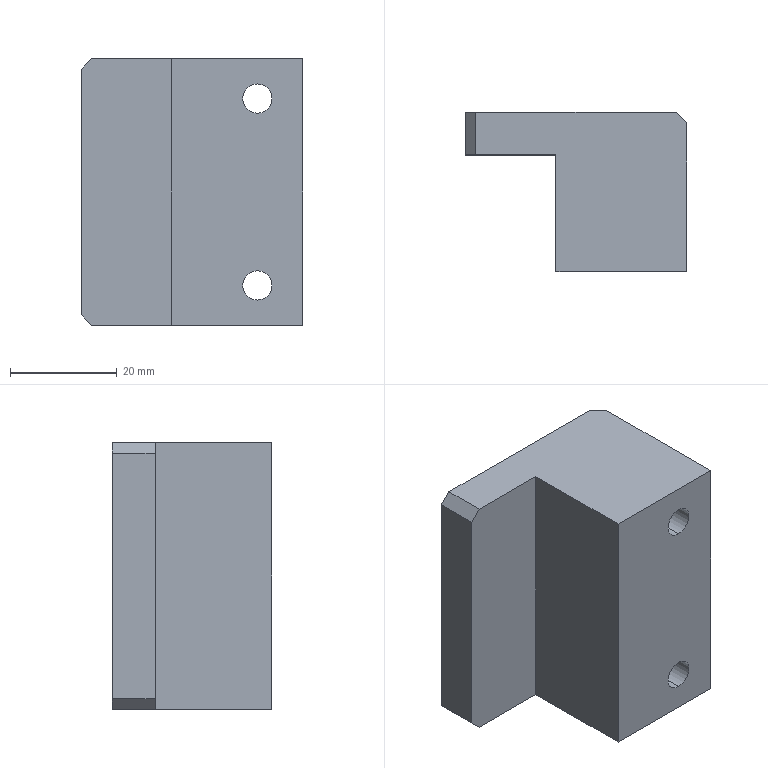Part | STEP file | PN_0006 Default | 1 solid | 21 faces | box 41.5 x 29.8 x 50 mm | volume 40902 mm3 | plane 13 | cylinder 8 | commonest cylinder face diameters 5.5 x4 11 x4
STEP:
#1=CARTESIAN_POINT('',(-8.5,23.8,2.));
#2=VERTEX_POINT('',#1);
#3=CARTESIAN_POINT('',(-8.5,23.8,13.));
#4=VERTEX_POINT('',#3);
#5=CARTESIAN_POINT('',(-8.5,23.8,7.5));
#6=DIRECTION('',(0.,1.,0.));
#7=DIRECTION('',(0.,0.,1.));
#8=AXIS2_PLACEMENT_3D('',#5,#6,#7);
#9=CIRCLE('',#8,5.5);
#10=EDGE_CURVE('',#2,#4,#9,.T.);
#11=ORIENTED_EDGE('',*,*,#10,.F.);
#12=CARTESIAN_POINT('',(-8.5,29.8,2.));
#13=VERTEX_POINT('',#12);
#14=CARTESIAN_POINT('',(-8.5,29.8,2.));
#15=DIRECTION('',(0.,1.,0.));
#16=VECTOR('',#15,1000.);
#17=LINE('',#14,#16);
#18=EDGE_CURVE('',#2,#13,#17,.T.);
#19=ORIENTED_EDGE('',*,*,#18,.T.);
#20=CARTESIAN_POINT('',(-8.5,29.8,13.));
#21=VERTEX_POINT('',#20);
#22=CARTESIAN_POINT('',(-8.5,29.8,7.5));
#23=DIRECTION('',(0.,1.,0.));
#24=DIRECTION('',(0.,0.,1.));
#25=AXIS2_PLACEMENT_3D('',#22,#23,#24);
#26=CIRCLE('',#25,5.5);
#27=EDGE_CURVE('',#13,#21,#26,.T.);
#28=ORIENTED_EDGE('',*,*,#27,.T.);
#29=CARTESIAN_POINT('',(-8.5,29.8,13.));
#30=DIRECTION('',(0.,1.,0.));
#31=VECTOR('',#30,1000.);
#32=LINE('',#29,#31);
#33=EDGE_CURVE('',#4,#21,#32,.T.);
#34=ORIENTED_EDGE('',*,*,#33,.F.);
#35=EDGE_LOOP('',(#11,#19,#28,#34));
#36=FACE_OUTER_BOUND('',#35,.T.);
#37=CARTESIAN_POINT('',(-8.5,29.8,7.5));
#38=DIRECTION('',(0.,1.,0.));
#39=DIRECTION('',(0.,0.,1.));
#40=AXIS2_PLACEMENT_3D('',#37,#38,#39);
#41=CYLINDRICAL_SURFACE('',#40,5.5);
#42=ADVANCED_FACE('',(#36),#41,.F.);
#43=CARTESIAN_POINT('',(-8.5,0.,4.75));
#44=VERTEX_POINT('',#43);
#45=CARTESIAN_POINT('',(-8.5,0.,10.25));
#46=VERTEX_POINT('',#45);
#47=CARTESIAN_POINT('',(-8.5,0.,7.5));
#48=DIRECTION('',(0.,1.,0.));
#49=DIRECTION('',(0.,0.,1.));
#50=AXIS2_PLACEMENT_3D('',#47,#48,#49);
#51=CIRCLE('',#50,2.75);
#52=EDGE_CURVE('',#44,#46,#51,.T.);
#53=ORIENTED_EDGE('',*,*,#52,.F.);
#54=CARTESIAN_POINT('',(-8.5,23.8,4.75));
#55=VERTEX_POINT('',#54);
#56=CARTESIAN_POINT('',(-8.5,29.8,4.75));
#57=DIRECTION('',(0.,1.,0.));
#58=VECTOR('',#57,1000.);
#59=LINE('',#56,#58);
#60=EDGE_CURVE('',#44,#55,#59,.T.);
#61=ORIENTED_EDGE('',*,*,#60,.T.);
#62=CARTESIAN_POINT('',(-8.5,23.8,10.25));
#63=VERTEX_POINT('',#62);
#64=CARTESIAN_POINT('',(-8.5,23.8,7.5));
#65=DIRECTION('',(0.,1.,0.));
#66=DIRECTION('',(0.,0.,1.));
#67=AXIS2_PLACEMENT_3D('',#64,#65,#66);
#68=CIRCLE('',#67,2.75);
#69=EDGE_CURVE('',#55,#63,#68,.T.);
#70=ORIENTED_EDGE('',*,*,#69,.T.);
#71=CARTESIAN_POINT('',(-8.5,29.8,10.25));
#72=DIRECTION('',(0.,1.,0.));
#73=VECTOR('',#72,1000.);
#74=LINE('',#71,#73);
#75=EDGE_CURVE('',#46,#63,#74,.T.);
#76=ORIENTED_EDGE('',*,*,#75,.F.);
#77=EDGE_LOOP('',(#53,#61,#70,#76));
#78=FACE_OUTER_BOUND('',#77,.T.);
#79=CARTESIAN_POINT('',(-8.5,29.8,7.5));
#80=DIRECTION('',(0.,1.,0.));
#81=DIRECTION('',(0.,0.,1.));
#82=AXIS2_PLACEMENT_3D('',#79,#80,#81);
#83=CYLINDRICAL_SURFACE('',#82,2.75);
#84=ADVANCED_FACE('',(#78),#83,.F.);
#85=CARTESIAN_POINT('',(-8.5,23.8,37.));
#86=VERTEX_POINT('',#85);
#87=CARTESIAN_POINT('',(-8.5,23.8,48.));
#88=VERTEX_POINT('',#87);
#89=CARTESIAN_POINT('',(-8.5,23.8,42.5));
#90=DIRECTION('',(0.,1.,0.));
#91=DIRECTION('',(0.,0.,1.));
#92=AXIS2_PLACEMENT_3D('',#89,#90,#91);
#93=CIRCLE('',#92,5.5);
#94=EDGE_CURVE('',#86,#88,#93,.T.);
#95=ORIENTED_EDGE('',*,*,#94,.F.);
#96=CARTESIAN_POINT('',(-8.5,29.8,37.));
#97=VERTEX_POINT('',#96);
#98=CARTESIAN_POINT('',(-8.5,29.8,37.));
#99=DIRECTION('',(0.,1.,0.));
#100=VECTOR('',#99,1000.);
#101=LINE('',#98,#100);
#102=EDGE_CURVE('',#86,#97,#101,.T.);
#103=ORIENTED_EDGE('',*,*,#102,.T.);
#104=CARTESIAN_POINT('',(-8.5,29.8,48.));
#105=VERTEX_POINT('',#104);
#106=CARTESIAN_POINT('',(-8.5,29.8,42.5));
#107=DIRECTION('',(0.,1.,0.));
#108=DIRECTION('',(0.,0.,1.));
#109=AXIS2_PLACEMENT_3D('',#106,#107,#108);
#110=CIRCLE('',#109,5.5);
#111=EDGE_CURVE('',#97,#105,#110,.T.);
#112=ORIENTED_EDGE('',*,*,#111,.T.);
#113=CARTESIAN_POINT('',(-8.5,29.8,48.));
#114=DIRECTION('',(0.,1.,0.));
#115=VECTOR('',#114,1000.);
#116=LINE('',#113,#115);
#117=EDGE_CURVE('',#88,#105,#116,.T.);
#118=ORIENTED_EDGE('',*,*,#117,.F.);
#119=EDGE_LOOP('',(#95,#103,#112,#118));
#120=FACE_OUTER_BOUND('',#119,.T.);
#121=CARTESIAN_POINT('',(-8.5,29.8,42.5));
#122=DIRECTION('',(0.,1.,0.));
#123=DIRECTION('',(0.,0.,1.));
#124=AXIS2_PLACEMENT_3D('',#121,#122,#123);
#125=CYLINDRICAL_SURFACE('',#124,5.5);
#126=ADVANCED_FACE('',(#120),#125,.F.);
#127=CARTESIAN_POINT('',(-8.5,0.,39.75));
#128=VERTEX_POINT('',#127);
#129=CARTESIAN_POINT('',(-8.5,0.,45.25));
#130=VERTEX_POINT('',#129);
#131=CARTESIAN_POINT('',(-8.5,0.,42.5));
#132=DIRECTION('',(0.,1.,0.));
#133=DIRECTION('',(0.,0.,1.));
#134=AXIS2_PLACEMENT_3D('',#131,#132,#133);
#135=CIRCLE('',#134,2.75);
#136=EDGE_CURVE('',#128,#130,#135,.T.);
#137=ORIENTED_EDGE('',*,*,#136,.F.);
#138=CARTESIAN_POINT('',(-8.5,23.8,39.75));
#139=VERTEX_POINT('',#138);
#140=CARTESIAN_POINT('',(-8.5,29.8,39.75));
#141=DIRECTION('',(0.,1.,0.));
#142=VECTOR('',#141,1000.);
#143=LINE('',#140,#142);
#144=EDGE_CURVE('',#128,#139,#143,.T.);
#145=ORIENTED_EDGE('',*,*,#144,.T.);
#146=CARTESIAN_POINT('',(-8.5,23.8,45.25));
#147=VERTEX_POINT('',#146);
#148=CARTESIAN_POINT('',(-8.5,23.8,42.5));
#149=DIRECTION('',(0.,1.,0.));
#150=DIRECTION('',(0.,0.,1.));
#151=AXIS2_PLACEMENT_3D('',#148,#149,#150);
#152=CIRCLE('',#151,2.75);
#153=EDGE_CURVE('',#139,#147,#152,.T.);
#154=ORIENTED_EDGE('',*,*,#153,.T.);
#155=CARTESIAN_POINT('',(-8.5,29.8,45.25));
#156=DIRECTION('',(0.,1.,0.));
#157=VECTOR('',#156,1000.);
#158=LINE('',#155,#157);
#159=EDGE_CURVE('',#130,#147,#158,.T.);
#160=ORIENTED_EDGE('',*,*,#159,.F.);
#161=EDGE_LOOP('',(#137,#145,#154,#160));
#162=FACE_OUTER_BOUND('',#161,.T.);
#163=CARTESIAN_POINT('',(-8.5,29.8,42.5));
#164=DIRECTION('',(0.,1.,0.));
#165=DIRECTION('',(0.,0.,1.));
#166=AXIS2_PLACEMENT_3D('',#163,#164,#165);
#167=CYLINDRICAL_SURFACE('',#166,2.75);
#168=ADVANCED_FACE('',(#162),#167,.F.);
#169=CARTESIAN_POINT('',(-41.5,29.8,48.));
#170=VERTEX_POINT('',#169);
#171=CARTESIAN_POINT('',(-41.5,29.8,2.));
#172=VERTEX_POINT('',#171);
#173=CARTESIAN_POINT('',(-41.5,29.8,50.));
#174=DIRECTION('',(0.,0.,-1.));
#175=VECTOR('',#174,1000.);
#176=LINE('',#173,#175);
#177=EDGE_CURVE('',#170,#172,#176,.T.);
#178=ORIENTED_EDGE('',*,*,#177,.T.);
#179=CARTESIAN_POINT('',(-41.5,21.8,2.));
#180=VERTEX_POINT('',#179);
#181=CARTESIAN_POINT('',(-41.5,21.8,2.));
#182=DIRECTION('',(0.,-1.,0.));
#183=VECTOR('',#182,1000.);
#184=LINE('',#181,#183);
#185=EDGE_CURVE('',#172,#180,#184,.T.);
#186=ORIENTED_EDGE('',*,*,#185,.T.);
#187=CARTESIAN_POINT('',(-41.5,21.8,48.));
#188=VERTEX_POINT('',#187);
#189=CARTESIAN_POINT('',(-41.5,21.8,50.));
#190=DIRECTION('',(0.,0.,-1.));
#191=VECTOR('',#190,1000.);
#192=LINE('',#189,#191);
#193=EDGE_CURVE('',#188,#180,#192,.T.);
#194=ORIENTED_EDGE('',*,*,#193,.F.);
#195=CARTESIAN_POINT('',(-41.5,21.8,48.));
#196=DIRECTION('',(0.,1.,0.));
#197=VECTOR('',#196,1000.);
#198=LINE('',#195,#197);
#199=EDGE_CURVE('',#188,#170,#198,.T.);
#200=ORIENTED_EDGE('',*,*,#199,.T.);
#201=EDGE_LOOP('',(#178,#186,#194,#200));
#202=FACE_OUTER_BOUND('',#201,.T.);
#203=CARTESIAN_POINT('',(-41.5,21.8,50.));
#204=DIRECTION('',(1.,0.,0.));
#205=DIRECTION('',(0.,0.,-1.));
#206=AXIS2_PLACEMENT_3D('',#203,#204,#205);
#207=PLANE('',#206);
#208=ADVANCED_FACE('',(#202),#207,.F.);
#209=ORIENTED_EDGE('',*,*,#193,.T.);
#210=CARTESIAN_POINT('',(-39.5,21.8,0.));
#211=VERTEX_POINT('',#210);
#212=CARTESIAN_POINT('',(-41.5,21.8,2.));
#213=DIRECTION('',(0.7071,0.,-0.7071));
#214=VECTOR('',#213,1000.);
#215=LINE('',#212,#214);
#216=EDGE_CURVE('',#180,#211,#215,.T.);
#217=ORIENTED_EDGE('',*,*,#216,.T.);
#218=CARTESIAN_POINT('',(-24.5,21.8,0.));
#219=VERTEX_POINT('',#218);
#220=CARTESIAN_POINT('',(-24.5,21.8,0.));
#221=DIRECTION('',(1.,0.,0.));
#222=VECTOR('',#221,1000.);
#223=LINE('',#220,#222);
#224=EDGE_CURVE('',#211,#219,#223,.T.);
#225=ORIENTED_EDGE('',*,*,#224,.T.);
#226=CARTESIAN_POINT('',(-24.5,21.8,50.));
#227=VERTEX_POINT('',#226);
#228=CARTESIAN_POINT('',(-24.5,21.8,50.));
#229=DIRECTION('',(0.,0.,-1.));
#230=VECTOR('',#229,1000.);
#231=LINE('',#228,#230);
#232=EDGE_CURVE('',#227,#219,#231,.T.);
#233=ORIENTED_EDGE('',*,*,#232,.F.);
#234=CARTESIAN_POINT('',(-39.5,21.8,50.));
#235=VERTEX_POINT('',#234);
#236=CARTESIAN_POINT('',(-24.5,21.8,50.));
#237=DIRECTION('',(1.,0.,0.));
#238=VECTOR('',#237,1000.);
#239=LINE('',#236,#238);
#240=EDGE_CURVE('',#235,#227,#239,.T.);
#241=ORIENTED_EDGE('',*,*,#240,.F.);
#242=CARTESIAN_POINT('',(-39.5,21.8,50.));
#243=DIRECTION('',(-0.7071,0.,-0.7071));
#244=VECTOR('',#243,1000.);
#245=LINE('',#242,#244);
#246=EDGE_CURVE('',#235,#188,#245,.T.);
#247=ORIENTED_EDGE('',*,*,#246,.T.);
#248=EDGE_LOOP('',(#209,#217,#225,#233,#241,#247));
#249=FACE_OUTER_BOUND('',#248,.T.);
#250=CARTESIAN_POINT('',(-24.5,21.8,50.));
#251=DIRECTION('',(0.,1.,0.));
#252=DIRECTION('',(0.,0.,1.));
#253=AXIS2_PLACEMENT_3D('',#250,#251,#252);
#254=PLANE('',#253);
#255=ADVANCED_FACE('',(#249),#254,.F.);
#256=CARTESIAN_POINT('',(-24.5,0.,0.));
#257=VERTEX_POINT('',#256);
#258=CARTESIAN_POINT('',(-24.5,0.,0.));
#259=DIRECTION('',(0.,-1.,0.));
#260=VECTOR('',#259,1000.);
#261=LINE('',#258,#260);
#262=EDGE_CURVE('',#219,#257,#261,.T.);
#263=ORIENTED_EDGE('',*,*,#262,.T.);
#264=CARTESIAN_POINT('',(-24.5,0.,50.));
#265=VERTEX_POINT('',#264);
#266=CARTESIAN_POINT('',(-24.5,0.,50.));
#267=DIRECTION('',(0.,0.,-1.));
#268=VECTOR('',#267,1000.);
#269=LINE('',#266,#268);
#270=EDGE_CURVE('',#265,#257,#269,.T.);
#271=ORIENTED_EDGE('',*,*,#270,.F.);
#272=CARTESIAN_POINT('',(-24.5,0.,50.));
#273=DIRECTION('',(0.,-1.,0.));
#274=VECTOR('',#273,1000.);
#275=LINE('',#272,#274);
#276=EDGE_CURVE('',#227,#265,#275,.T.);
#277=ORIENTED_EDGE('',*,*,#276,.F.);
#278=ORIENTED_EDGE('',*,*,#232,.T.);
#279=EDGE_LOOP('',(#263,#271,#277,#278));
#280=FACE_OUTER_BOUND('',#279,.T.);
#281=CARTESIAN_POINT('',(-24.5,0.,50.));
#282=DIRECTION('',(1.,0.,0.));
#283=DIRECTION('',(0.,0.,-1.));
#284=AXIS2_PLACEMENT_3D('',#281,#282,#283);
#285=PLANE('',#284);
#286=ADVANCED_FACE('',(#280),#285,.F.);
#287=CARTESIAN_POINT('',(-8.5,0.,7.5));
#288=DIRECTION('',(0.,1.,0.));
#289=DIRECTION('',(0.,0.,1.));
#290=AXIS2_PLACEMENT_3D('',#287,#288,#289);
#291=CIRCLE('',#290,2.75);
#292=EDGE_CURVE('',#46,#44,#291,.T.);
#293=ORIENTED_EDGE('',*,*,#292,.T.);
#294=ORIENTED_EDGE('',*,*,#52,.T.);
#295=EDGE_LOOP('',(#293,#294));
#296=FACE_BOUND('',#295,.T.);
#297=CARTESIAN_POINT('',(-8.5,0.,42.5));
#298=DIRECTION('',(0.,1.,0.));
#299=DIRECTION('',(0.,0.,1.));
#300=AXIS2_PLACEMENT_3D('',#297,#298,#299);
#301=CIRCLE('',#300,2.75);
#302=EDGE_CURVE('',#130,#128,#301,.T.);
#303=ORIENTED_EDGE('',*,*,#302,.T.);
#304=ORIENTED_EDGE('',*,*,#136,.T.);
#305=EDGE_LOOP('',(#303,#304));
#306=FACE_BOUND('',#305,.T.);
#307=CARTESIAN_POINT('',(0.,0.,0.));
#308=VERTEX_POINT('',#307);
#309=CARTESIAN_POINT('',(0.,0.,0.));
#310=DIRECTION('',(1.,0.,0.));
#311=VECTOR('',#310,1000.);
#312=LINE('',#309,#311);
#313=EDGE_CURVE('',#257,#308,#312,.T.);
#314=ORIENTED_EDGE('',*,*,#313,.T.);
#315=CARTESIAN_POINT('',(0.,0.,50.));
#316=VERTEX_POINT('',#315);
#317=CARTESIAN_POINT('',(0.,0.,50.));
#318=DIRECTION('',(0.,0.,-1.));
#319=VECTOR('',#318,1000.);
#320=LINE('',#317,#319);
#321=EDGE_CURVE('',#316,#308,#320,.T.);
#322=ORIENTED_EDGE('',*,*,#321,.F.);
#323=CARTESIAN_POINT('',(0.,0.,50.));
#324=DIRECTION('',(1.,0.,0.));
#325=VECTOR('',#324,1000.);
#326=LINE('',#323,#325);
#327=EDGE_CURVE('',#265,#316,#326,.T.);
#328=ORIENTED_EDGE('',*,*,#327,.F.);
#329=ORIENTED_EDGE('',*,*,#270,.T.);
#330=EDGE_LOOP('',(#314,#322,#328,#329));
#331=FACE_OUTER_BOUND('',#330,.T.);
#332=CARTESIAN_POINT('',(0.,0.,50.));
#333=DIRECTION('',(0.,1.,0.));
#334=DIRECTION('',(-1.,0.,0.));
#335=AXIS2_PLACEMENT_3D('',#332,#333,#334);
#336=PLANE('',#335);
#337=ADVANCED_FACE('',(#296,#306,#331),#336,.F.);
#338=CARTESIAN_POINT('',(0.,27.8,0.));
#339=VERTEX_POINT('',#338);
#340=CARTESIAN_POINT('',(0.,29.8,0.));
#341=DIRECTION('',(0.,1.,0.));
#342=VECTOR('',#341,1000.);
#343=LINE('',#340,#342);
#344=EDGE_CURVE('',#308,#339,#343,.T.);
#345=ORIENTED_EDGE('',*,*,#344,.T.);
#346=CARTESIAN_POINT('',(0.,27.8,50.));
#347=VERTEX_POINT('',#346);
#348=CARTESIAN_POINT('',(0.,27.8,50.));
#349=DIRECTION('',(0.,0.,1.));
#350=VECTOR('',#349,1000.);
#351=LINE('',#348,#350);
#352=EDGE_CURVE('',#339,#347,#351,.T.);
#353=ORIENTED_EDGE('',*,*,#352,.T.);
#354=CARTESIAN_POINT('',(0.,29.8,50.));
#355=DIRECTION('',(0.,1.,0.));
#356=VECTOR('',#355,1000.);
#357=LINE('',#354,#356);
#358=EDGE_CURVE('',#316,#347,#357,.T.);
#359=ORIENTED_EDGE('',*,*,#358,.F.);
#360=ORIENTED_EDGE('',*,*,#321,.T.);
#361=EDGE_LOOP('',(#345,#353,#359,#360));
#362=FACE_OUTER_BOUND('',#361,.T.);
#363=CARTESIAN_POINT('',(0.,29.8,50.));
#364=DIRECTION('',(-1.,0.,0.));
#365=DIRECTION('',(0.,-1.,0.));
#366=AXIS2_PLACEMENT_3D('',#363,#364,#365);
#367=PLANE('',#366);
#368=ADVANCED_FACE('',(#362),#367,.F.);
#369=CARTESIAN_POINT('',(-8.5,29.8,7.5));
#370=DIRECTION('',(0.,1.,0.));
#371=DIRECTION('',(0.,0.,1.));
#372=AXIS2_PLACEMENT_3D('',#369,#370,#371);
#373=CIRCLE('',#372,5.5);
#374=EDGE_CURVE('',#21,#13,#373,.T.);
#375=ORIENTED_EDGE('',*,*,#374,.F.);
#376=ORIENTED_EDGE('',*,*,#27,.F.);
#377=EDGE_LOOP('',(#375,#376));
#378=FACE_BOUND('',#377,.T.);
#379=CARTESIAN_POINT('',(-8.5,29.8,42.5));
#380=DIRECTION('',(0.,1.,0.));
#381=DIRECTION('',(0.,0.,1.));
#382=AXIS2_PLACEMENT_3D('',#379,#380,#381);
#383=CIRCLE('',#382,5.5);
#384=EDGE_CURVE('',#105,#97,#383,.T.);
#385=ORIENTED_EDGE('',*,*,#384,.F.);
#386=ORIENTED_EDGE('',*,*,#111,.F.);
#387=EDGE_LOOP('',(#385,#386));
#388=FACE_BOUND('',#387,.T.);
#389=CARTESIAN_POINT('',(-2.,29.8,0.));
#390=VERTEX_POINT('',#389);
#391=CARTESIAN_POINT('',(-39.5,29.8,0.));
#392=VERTEX_POINT('',#391);
#393=CARTESIAN_POINT('',(-41.5,29.8,0.));
#394=DIRECTION('',(-1.,0.,0.));
#395=VECTOR('',#394,1000.);
#396=LINE('',#393,#395);
#397=EDGE_CURVE('',#390,#392,#396,.T.);
#398=ORIENTED_EDGE('',*,*,#397,.T.);
#399=CARTESIAN_POINT('',(-41.5,29.8,2.));
#400=DIRECTION('',(-0.7071,0.,0.7071));
#401=VECTOR('',#400,1000.);
#402=LINE('',#399,#401);
#403=EDGE_CURVE('',#392,#172,#402,.T.);
#404=ORIENTED_EDGE('',*,*,#403,.T.);
#405=ORIENTED_EDGE('',*,*,#177,.F.);
#406=CARTESIAN_POINT('',(-39.5,29.8,50.));
#407=VERTEX_POINT('',#406);
#408=CARTESIAN_POINT('',(-39.5,29.8,50.));
#409=DIRECTION('',(0.7071,0.,0.7071));
#410=VECTOR('',#409,1000.);
#411=LINE('',#408,#410);
#412=EDGE_CURVE('',#170,#407,#411,.T.);
#413=ORIENTED_EDGE('',*,*,#412,.T.);
#414=CARTESIAN_POINT('',(-2.,29.8,50.));
#415=VERTEX_POINT('',#414);
#416=CARTESIAN_POINT('',(-41.5,29.8,50.));
#417=DIRECTION('',(-1.,0.,0.));
#418=VECTOR('',#417,1000.);
#419=LINE('',#416,#418);
#420=EDGE_CURVE('',#415,#407,#419,.T.);
#421=ORIENTED_EDGE('',*,*,#420,.F.);
#422=CARTESIAN_POINT('',(-2.,29.8,50.));
#423=DIRECTION('',(0.,0.,-1.));
#424=VECTOR('',#423,1000.);
#425=LINE('',#422,#424);
#426=EDGE_CURVE('',#415,#390,#425,.T.);
#427=ORIENTED_EDGE('',*,*,#426,.T.);
#428=EDGE_LOOP('',(#398,#404,#405,#413,#421,#427));
#429=FACE_OUTER_BOUND('',#428,.T.);
#430=CARTESIAN_POINT('',(-41.5,29.8,50.));
#431=DIRECTION('',(0.,-1.,0.));
#432=DIRECTION('',(0.,0.,-1.));
#433=AXIS2_PLACEMENT_3D('',#430,#431,#432);
#434=PLANE('',#433);
#435=ADVANCED_FACE('',(#378,#388,#429),#434,.F.);
#436=ORIENTED_EDGE('',*,*,#420,.T.);
#437=CARTESIAN_POINT('',(-39.5,0.,50.));
#438=DIRECTION('',(0.,-1.,0.));
#439=VECTOR('',#438,1000.);
#440=LINE('',#437,#439);
#441=EDGE_CURVE('',#407,#235,#440,.T.);
#442=ORIENTED_EDGE('',*,*,#441,.T.);
#443=ORIENTED_EDGE('',*,*,#240,.T.);
#444=ORIENTED_EDGE('',*,*,#276,.T.);
#445=ORIENTED_EDGE('',*,*,#327,.T.);
#446=ORIENTED_EDGE('',*,*,#358,.T.);
#447=CARTESIAN_POINT('',(-2.,29.8,50.));
#448=DIRECTION('',(-0.7071,0.7071,0.));
#449=VECTOR('',#448,1000.);
#450=LINE('',#447,#449);
#451=EDGE_CURVE('',#347,#415,#450,.T.);
#452=ORIENTED_EDGE('',*,*,#451,.T.);
#453=EDGE_LOOP('',(#436,#442,#443,#444,#445,#446,#452));
#454=FACE_OUTER_BOUND('',#453,.T.);
#455=CARTESIAN_POINT('',(0.,0.,50.));
#456=DIRECTION('',(0.,0.,-1.));
#457=DIRECTION('',(-1.,0.,0.));
#458=AXIS2_PLACEMENT_3D('',#455,#456,#457);
#459=PLANE('',#458);
#460=ADVANCED_FACE('',(#454),#459,.F.);
#461=ORIENTED_EDGE('',*,*,#224,.F.);
#462=CARTESIAN_POINT('',(-39.5,29.8,0.));
#463=DIRECTION('',(0.,1.,0.));
#464=VECTOR('',#463,1000.);
#465=LINE('',#462,#464);
#466=EDGE_CURVE('',#211,#392,#465,.T.);
#467=ORIENTED_EDGE('',*,*,#466,.T.);
#468=ORIENTED_EDGE('',*,*,#397,.F.);
#469=CARTESIAN_POINT('',(13.9,13.9,0.));
#470=DIRECTION('',(0.7071,-0.7071,0.));
#471=VECTOR('',#470,1000.);
#472=LINE('',#469,#471);
#473=EDGE_CURVE('',#390,#339,#472,.T.);
#474=ORIENTED_EDGE('',*,*,#473,.T.);
#475=ORIENTED_EDGE('',*,*,#344,.F.);
#476=ORIENTED_EDGE('',*,*,#313,.F.);
#477=ORIENTED_EDGE('',*,*,#262,.F.);
#478=EDGE_LOOP('',(#461,#467,#468,#474,#475,#476,#477));
#479=FACE_OUTER_BOUND('',#478,.T.);
#480=CARTESIAN_POINT('',(0.,0.,0.));
#481=DIRECTION('',(0.,0.,-1.));
#482=DIRECTION('',(-1.,0.,0.));
#483=AXIS2_PLACEMENT_3D('',#480,#481,#482);
#484=PLANE('',#483);
#485=ADVANCED_FACE('',(#479),#484,.T.);
#486=ORIENTED_EDGE('',*,*,#403,.F.);
#487=ORIENTED_EDGE('',*,*,#466,.F.);
#488=ORIENTED_EDGE('',*,*,#216,.F.);
#489=ORIENTED_EDGE('',*,*,#185,.F.);
#490=EDGE_LOOP('',(#486,#487,#488,#489));
#491=FACE_OUTER_BOUND('',#490,.T.);
#492=CARTESIAN_POINT('',(-41.5,21.8,2.));
#493=DIRECTION('',(-0.7071,0.,-0.7071));
#494=DIRECTION('',(0.,1.,0.));
#495=AXIS2_PLACEMENT_3D('',#492,#493,#494);
#496=PLANE('',#495);
#497=ADVANCED_FACE('',(#491),#496,.T.);
#498=ORIENTED_EDGE('',*,*,#412,.F.);
#499=ORIENTED_EDGE('',*,*,#199,.F.);
#500=ORIENTED_EDGE('',*,*,#246,.F.);
#501=ORIENTED_EDGE('',*,*,#441,.F.);
#502=EDGE_LOOP('',(#498,#499,#500,#501));
#503=FACE_OUTER_BOUND('',#502,.T.);
#504=CARTESIAN_POINT('',(-39.5,0.,50.));
#505=DIRECTION('',(0.7071,0.,-0.7071));
#506=DIRECTION('',(0.,-1.,0.));
#507=AXIS2_PLACEMENT_3D('',#504,#505,#506);
#508=PLANE('',#507);
#509=ADVANCED_FACE('',(#503),#508,.F.);
#510=ORIENTED_EDGE('',*,*,#451,.F.);
#511=ORIENTED_EDGE('',*,*,#352,.F.);
#512=ORIENTED_EDGE('',*,*,#473,.F.);
#513=ORIENTED_EDGE('',*,*,#426,.F.);
#514=EDGE_LOOP('',(#510,#511,#512,#513));
#515=FACE_OUTER_BOUND('',#514,.T.);
#516=CARTESIAN_POINT('',(-2.,29.8,50.));
#517=DIRECTION('',(-0.7071,-0.7071,0.));
#518=DIRECTION('',(0.,0.,-1.));
#519=AXIS2_PLACEMENT_3D('',#516,#517,#518);
#520=PLANE('',#519);
#521=ADVANCED_FACE('',(#515),#520,.F.);
#522=ORIENTED_EDGE('',*,*,#144,.F.);
#523=ORIENTED_EDGE('',*,*,#302,.F.);
#524=ORIENTED_EDGE('',*,*,#159,.T.);
#525=CARTESIAN_POINT('',(-8.5,23.8,42.5));
#526=DIRECTION('',(0.,1.,0.));
#527=DIRECTION('',(0.,0.,1.));
#528=AXIS2_PLACEMENT_3D('',#525,#526,#527);
#529=CIRCLE('',#528,2.75);
#530=EDGE_CURVE('',#147,#139,#529,.T.);
#531=ORIENTED_EDGE('',*,*,#530,.T.);
#532=EDGE_LOOP('',(#522,#523,#524,#531));
#533=FACE_OUTER_BOUND('',#532,.T.);
#534=CARTESIAN_POINT('',(-8.5,29.8,42.5));
#535=DIRECTION('',(0.,1.,0.));
#536=DIRECTION('',(0.,0.,1.));
#537=AXIS2_PLACEMENT_3D('',#534,#535,#536);
#538=CYLINDRICAL_SURFACE('',#537,2.75);
#539=ADVANCED_FACE('',(#533),#538,.F.);
#540=ORIENTED_EDGE('',*,*,#530,.F.);
#541=ORIENTED_EDGE('',*,*,#153,.F.);
#542=EDGE_LOOP('',(#540,#541));
#543=FACE_BOUND('',#542,.T.);
#544=CARTESIAN_POINT('',(-8.5,23.8,42.5));
#545=DIRECTION('',(0.,1.,0.));
#546=DIRECTION('',(0.,0.,1.));
#547=AXIS2_PLACEMENT_3D('',#544,#545,#546);
#548=CIRCLE('',#547,5.5);
#549=EDGE_CURVE('',#88,#86,#548,.T.);
#550=ORIENTED_EDGE('',*,*,#549,.T.);
#551=ORIENTED_EDGE('',*,*,#94,.T.);
#552=EDGE_LOOP('',(#550,#551));
#553=FACE_OUTER_BOUND('',#552,.T.);
#554=CARTESIAN_POINT('',(-5.75,23.8,42.5));
#555=DIRECTION('',(0.,-1.,0.));
#556=DIRECTION('',(0.,0.,-1.));
#557=AXIS2_PLACEMENT_3D('',#554,#555,#556);
#558=PLANE('',#557);
#559=ADVANCED_FACE('',(#543,#553),#558,.F.);
#560=ORIENTED_EDGE('',*,*,#102,.F.);
#561=ORIENTED_EDGE('',*,*,#549,.F.);
#562=ORIENTED_EDGE('',*,*,#117,.T.);
#563=ORIENTED_EDGE('',*,*,#384,.T.);
#564=EDGE_LOOP('',(#560,#561,#562,#563));
#565=FACE_OUTER_BOUND('',#564,.T.);
#566=CARTESIAN_POINT('',(-8.5,29.8,42.5));
#567=DIRECTION('',(0.,1.,0.));
#568=DIRECTION('',(0.,0.,1.));
#569=AXIS2_PLACEMENT_3D('',#566,#567,#568);
#570=CYLINDRICAL_SURFACE('',#569,5.5);
#571=ADVANCED_FACE('',(#565),#570,.F.);
#572=ORIENTED_EDGE('',*,*,#60,.F.);
#573=ORIENTED_EDGE('',*,*,#292,.F.);
#574=ORIENTED_EDGE('',*,*,#75,.T.);
#575=CARTESIAN_POINT('',(-8.5,23.8,7.5));
#576=DIRECTION('',(0.,1.,0.));
#577=DIRECTION('',(0.,0.,1.));
#578=AXIS2_PLACEMENT_3D('',#575,#576,#577);
#579=CIRCLE('',#578,2.75);
#580=EDGE_CURVE('',#63,#55,#579,.T.);
#581=ORIENTED_EDGE('',*,*,#580,.T.);
#582=EDGE_LOOP('',(#572,#573,#574,#581));
#583=FACE_OUTER_BOUND('',#582,.T.);
#584=CARTESIAN_POINT('',(-8.5,29.8,7.5));
#585=DIRECTION('',(0.,1.,0.));
#586=DIRECTION('',(0.,0.,1.));
#587=AXIS2_PLACEMENT_3D('',#584,#585,#586);
#588=CYLINDRICAL_SURFACE('',#587,2.75);
#589=ADVANCED_FACE('',(#583),#588,.F.);
#590=ORIENTED_EDGE('',*,*,#580,.F.);
#591=ORIENTED_EDGE('',*,*,#69,.F.);
#592=EDGE_LOOP('',(#590,#591));
#593=FACE_BOUND('',#592,.T.);
#594=CARTESIAN_POINT('',(-8.5,23.8,7.5));
#595=DIRECTION('',(0.,1.,0.));
#596=DIRECTION('',(0.,0.,1.));
#597=AXIS2_PLACEMENT_3D('',#594,#595,#596);
#598=CIRCLE('',#597,5.5);
#599=EDGE_CURVE('',#4,#2,#598,.T.);
#600=ORIENTED_EDGE('',*,*,#599,.T.);
#601=ORIENTED_EDGE('',*,*,#10,.T.);
#602=EDGE_LOOP('',(#600,#601));
#603=FACE_OUTER_BOUND('',#602,.T.);
#604=CARTESIAN_POINT('',(-5.75,23.8,7.5));
#605=DIRECTION('',(0.,-1.,0.));
#606=DIRECTION('',(0.,0.,-1.));
#607=AXIS2_PLACEMENT_3D('',#604,#605,#606);
#608=PLANE('',#607);
#609=ADVANCED_FACE('',(#593,#603),#608,.F.);
#610=ORIENTED_EDGE('',*,*,#18,.F.);
#611=ORIENTED_EDGE('',*,*,#599,.F.);
#612=ORIENTED_EDGE('',*,*,#33,.T.);
#613=ORIENTED_EDGE('',*,*,#374,.T.);
#614=EDGE_LOOP('',(#610,#611,#612,#613));
#615=FACE_OUTER_BOUND('',#614,.T.);
#616=CARTESIAN_POINT('',(-8.5,29.8,7.5));
#617=DIRECTION('',(0.,1.,0.));
#618=DIRECTION('',(0.,0.,1.));
#619=AXIS2_PLACEMENT_3D('',#616,#617,#618);
#620=CYLINDRICAL_SURFACE('',#619,5.5);
#621=ADVANCED_FACE('',(#615),#620,.F.);
#622=CLOSED_SHELL('',(#42,#84,#126,#168,#208,#255,#286,#337,#368,#435,#460,#485,#497,#509,#521,#539,#559,#571,#589,#609,#621));
#623=MANIFOLD_SOLID_BREP('',#622);
#624=CARTESIAN_POINT('',(0.,0.,0.));
#625=DIRECTION('',(0.,0.,1.));
#626=DIRECTION('',(1.,0.,0.));
#627=AXIS2_PLACEMENT_3D('',#624,#625,#626);
#628=(LENGTH_UNIT()NAMED_UNIT(*)SI_UNIT(.MILLI.,.METRE.));
#629=UNCERTAINTY_MEASURE_WITH_UNIT(LENGTH_MEASURE(0.00001),#628,'','');
#630=(NAMED_UNIT(*)PLANE_ANGLE_UNIT()SI_UNIT($,.RADIAN.));
#631=(NAMED_UNIT(*)SI_UNIT($,.STERADIAN.)SOLID_ANGLE_UNIT());
#632=(GEOMETRIC_REPRESENTATION_CONTEXT(3)GLOBAL_UNCERTAINTY_ASSIGNED_CONTEXT((#629))GLOBAL_UNIT_ASSIGNED_CONTEXT((#628,#630,#631))REPRESENTATION_CONTEXT('',''));
#633=ADVANCED_BREP_SHAPE_REPRESENTATION('',(#623,#627),#632);